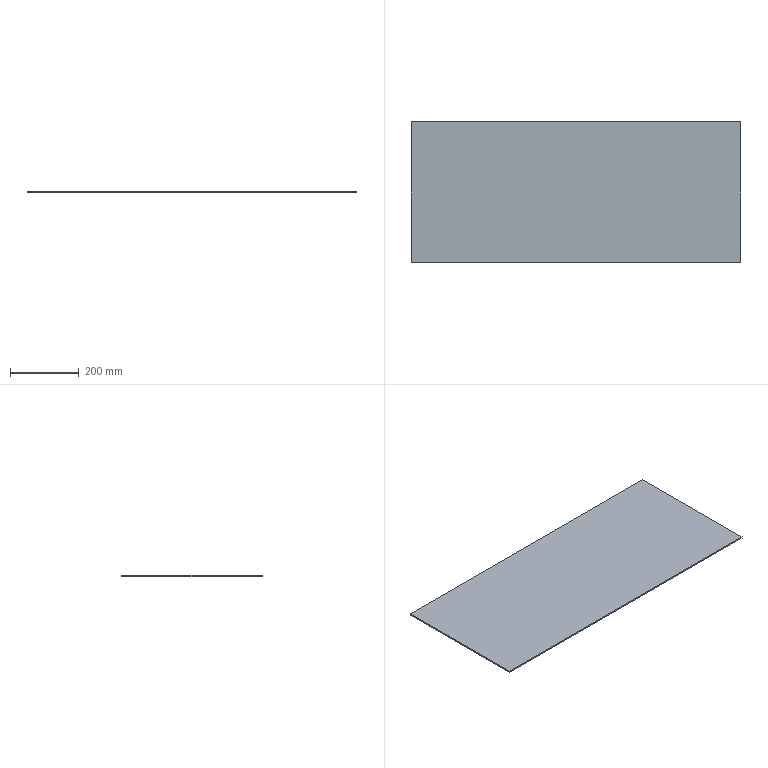Part | STEP file | X77-05601 | 1 solid | 6 faces | box 960 x 410 x 4 mm | volume 1574400 mm3 | plane 6
STEP:
#1=CARTESIAN_POINT('',(521.386,-150.547,0.));
#2=VERTEX_POINT('',#1);
#3=CARTESIAN_POINT('',(521.386,-560.547,0.));
#4=VERTEX_POINT('',#3);
#5=CARTESIAN_POINT('',(521.386,-560.547,0.));
#6=DIRECTION('',(0.,-1.,0.));
#7=VECTOR('',#6,1000.);
#8=LINE('',#5,#7);
#9=EDGE_CURVE('',#2,#4,#8,.T.);
#10=ORIENTED_EDGE('',*,*,#9,.T.);
#11=CARTESIAN_POINT('',(521.386,-560.547,4.));
#12=VERTEX_POINT('',#11);
#13=CARTESIAN_POINT('',(521.386,-560.547,4.));
#14=DIRECTION('',(0.,0.,-1.));
#15=VECTOR('',#14,1000.);
#16=LINE('',#13,#15);
#17=EDGE_CURVE('',#12,#4,#16,.T.);
#18=ORIENTED_EDGE('',*,*,#17,.F.);
#19=CARTESIAN_POINT('',(521.386,-150.547,4.));
#20=VERTEX_POINT('',#19);
#21=CARTESIAN_POINT('',(521.386,-560.547,4.));
#22=DIRECTION('',(0.,-1.,0.));
#23=VECTOR('',#22,1000.);
#24=LINE('',#21,#23);
#25=EDGE_CURVE('',#20,#12,#24,.T.);
#26=ORIENTED_EDGE('',*,*,#25,.F.);
#27=CARTESIAN_POINT('',(521.386,-150.547,4.));
#28=DIRECTION('',(0.,0.,-1.));
#29=VECTOR('',#28,1000.);
#30=LINE('',#27,#29);
#31=EDGE_CURVE('',#20,#2,#30,.T.);
#32=ORIENTED_EDGE('',*,*,#31,.T.);
#33=EDGE_LOOP('',(#10,#18,#26,#32));
#34=FACE_OUTER_BOUND('',#33,.T.);
#35=CARTESIAN_POINT('',(521.386,-560.547,4.));
#36=DIRECTION('',(1.,0.,0.));
#37=DIRECTION('',(0.,0.,-1.));
#38=AXIS2_PLACEMENT_3D('',#35,#36,#37);
#39=PLANE('',#38);
#40=ADVANCED_FACE('',(#34),#39,.F.);
#41=CARTESIAN_POINT('',(1481.386,-560.547,0.));
#42=VERTEX_POINT('',#41);
#43=CARTESIAN_POINT('',(521.386,-560.547,0.));
#44=DIRECTION('',(1.,0.,0.));
#45=VECTOR('',#44,1000.);
#46=LINE('',#43,#45);
#47=EDGE_CURVE('',#4,#42,#46,.T.);
#48=ORIENTED_EDGE('',*,*,#47,.T.);
#49=CARTESIAN_POINT('',(1481.386,-560.547,4.));
#50=VERTEX_POINT('',#49);
#51=CARTESIAN_POINT('',(1481.386,-560.547,4.));
#52=DIRECTION('',(0.,0.,-1.));
#53=VECTOR('',#52,1000.);
#54=LINE('',#51,#53);
#55=EDGE_CURVE('',#50,#42,#54,.T.);
#56=ORIENTED_EDGE('',*,*,#55,.F.);
#57=CARTESIAN_POINT('',(521.386,-560.547,4.));
#58=DIRECTION('',(1.,0.,0.));
#59=VECTOR('',#58,1000.);
#60=LINE('',#57,#59);
#61=EDGE_CURVE('',#12,#50,#60,.T.);
#62=ORIENTED_EDGE('',*,*,#61,.F.);
#63=ORIENTED_EDGE('',*,*,#17,.T.);
#64=EDGE_LOOP('',(#48,#56,#62,#63));
#65=FACE_OUTER_BOUND('',#64,.T.);
#66=CARTESIAN_POINT('',(521.386,-560.547,4.));
#67=DIRECTION('',(0.,1.,0.));
#68=DIRECTION('',(0.,0.,1.));
#69=AXIS2_PLACEMENT_3D('',#66,#67,#68);
#70=PLANE('',#69);
#71=ADVANCED_FACE('',(#65),#70,.F.);
#72=CARTESIAN_POINT('',(1481.386,-150.547,0.));
#73=VERTEX_POINT('',#72);
#74=CARTESIAN_POINT('',(1481.386,-560.547,0.));
#75=DIRECTION('',(0.,1.,0.));
#76=VECTOR('',#75,1000.);
#77=LINE('',#74,#76);
#78=EDGE_CURVE('',#42,#73,#77,.T.);
#79=ORIENTED_EDGE('',*,*,#78,.T.);
#80=CARTESIAN_POINT('',(1481.386,-150.547,4.));
#81=VERTEX_POINT('',#80);
#82=CARTESIAN_POINT('',(1481.386,-150.547,4.));
#83=DIRECTION('',(0.,0.,-1.));
#84=VECTOR('',#83,1000.);
#85=LINE('',#82,#84);
#86=EDGE_CURVE('',#81,#73,#85,.T.);
#87=ORIENTED_EDGE('',*,*,#86,.F.);
#88=CARTESIAN_POINT('',(1481.386,-560.547,4.));
#89=DIRECTION('',(0.,1.,0.));
#90=VECTOR('',#89,1000.);
#91=LINE('',#88,#90);
#92=EDGE_CURVE('',#50,#81,#91,.T.);
#93=ORIENTED_EDGE('',*,*,#92,.F.);
#94=ORIENTED_EDGE('',*,*,#55,.T.);
#95=EDGE_LOOP('',(#79,#87,#93,#94));
#96=FACE_OUTER_BOUND('',#95,.T.);
#97=CARTESIAN_POINT('',(1481.386,-560.547,4.));
#98=DIRECTION('',(-1.,0.,0.));
#99=DIRECTION('',(0.,0.,1.));
#100=AXIS2_PLACEMENT_3D('',#97,#98,#99);
#101=PLANE('',#100);
#102=ADVANCED_FACE('',(#96),#101,.F.);
#103=CARTESIAN_POINT('',(521.386,-150.547,0.));
#104=DIRECTION('',(-1.,0.,0.));
#105=VECTOR('',#104,1000.);
#106=LINE('',#103,#105);
#107=EDGE_CURVE('',#73,#2,#106,.T.);
#108=ORIENTED_EDGE('',*,*,#107,.T.);
#109=ORIENTED_EDGE('',*,*,#31,.F.);
#110=CARTESIAN_POINT('',(521.386,-150.547,4.));
#111=DIRECTION('',(-1.,0.,0.));
#112=VECTOR('',#111,1000.);
#113=LINE('',#110,#112);
#114=EDGE_CURVE('',#81,#20,#113,.T.);
#115=ORIENTED_EDGE('',*,*,#114,.F.);
#116=ORIENTED_EDGE('',*,*,#86,.T.);
#117=EDGE_LOOP('',(#108,#109,#115,#116));
#118=FACE_OUTER_BOUND('',#117,.T.);
#119=CARTESIAN_POINT('',(521.386,-150.547,4.));
#120=DIRECTION('',(0.,-1.,0.));
#121=DIRECTION('',(0.,0.,-1.));
#122=AXIS2_PLACEMENT_3D('',#119,#120,#121);
#123=PLANE('',#122);
#124=ADVANCED_FACE('',(#118),#123,.F.);
#125=ORIENTED_EDGE('',*,*,#25,.T.);
#126=ORIENTED_EDGE('',*,*,#61,.T.);
#127=ORIENTED_EDGE('',*,*,#92,.T.);
#128=ORIENTED_EDGE('',*,*,#114,.T.);
#129=EDGE_LOOP('',(#125,#126,#127,#128));
#130=FACE_OUTER_BOUND('',#129,.T.);
#131=CARTESIAN_POINT('',(521.386,-150.547,4.));
#132=DIRECTION('',(0.,0.,-1.));
#133=DIRECTION('',(-1.,0.,0.));
#134=AXIS2_PLACEMENT_3D('',#131,#132,#133);
#135=PLANE('',#134);
#136=ADVANCED_FACE('',(#130),#135,.F.);
#137=ORIENTED_EDGE('',*,*,#9,.F.);
#138=ORIENTED_EDGE('',*,*,#107,.F.);
#139=ORIENTED_EDGE('',*,*,#78,.F.);
#140=ORIENTED_EDGE('',*,*,#47,.F.);
#141=EDGE_LOOP('',(#137,#138,#139,#140));
#142=FACE_OUTER_BOUND('',#141,.T.);
#143=CARTESIAN_POINT('',(521.386,-150.547,0.));
#144=DIRECTION('',(0.,0.,-1.));
#145=DIRECTION('',(-1.,0.,0.));
#146=AXIS2_PLACEMENT_3D('',#143,#144,#145);
#147=PLANE('',#146);
#148=ADVANCED_FACE('',(#142),#147,.T.);
#149=CLOSED_SHELL('',(#40,#71,#102,#124,#136,#148));
#150=MANIFOLD_SOLID_BREP('',#149);
#151=CARTESIAN_POINT('',(0.,0.,0.));
#152=DIRECTION('',(0.,0.,1.));
#153=DIRECTION('',(1.,0.,0.));
#154=AXIS2_PLACEMENT_3D('',#151,#152,#153);
#155=(LENGTH_UNIT()NAMED_UNIT(*)SI_UNIT(.MILLI.,.METRE.));
#156=UNCERTAINTY_MEASURE_WITH_UNIT(LENGTH_MEASURE(0.00001),#155,'','');
#157=(NAMED_UNIT(*)PLANE_ANGLE_UNIT()SI_UNIT($,.RADIAN.));
#158=(NAMED_UNIT(*)SI_UNIT($,.STERADIAN.)SOLID_ANGLE_UNIT());
#159=(GEOMETRIC_REPRESENTATION_CONTEXT(3)GLOBAL_UNCERTAINTY_ASSIGNED_CONTEXT((#156))GLOBAL_UNIT_ASSIGNED_CONTEXT((#155,#157,#158))REPRESENTATION_CONTEXT('',''));
#160=ADVANCED_BREP_SHAPE_REPRESENTATION('',(#150,#154),#159);